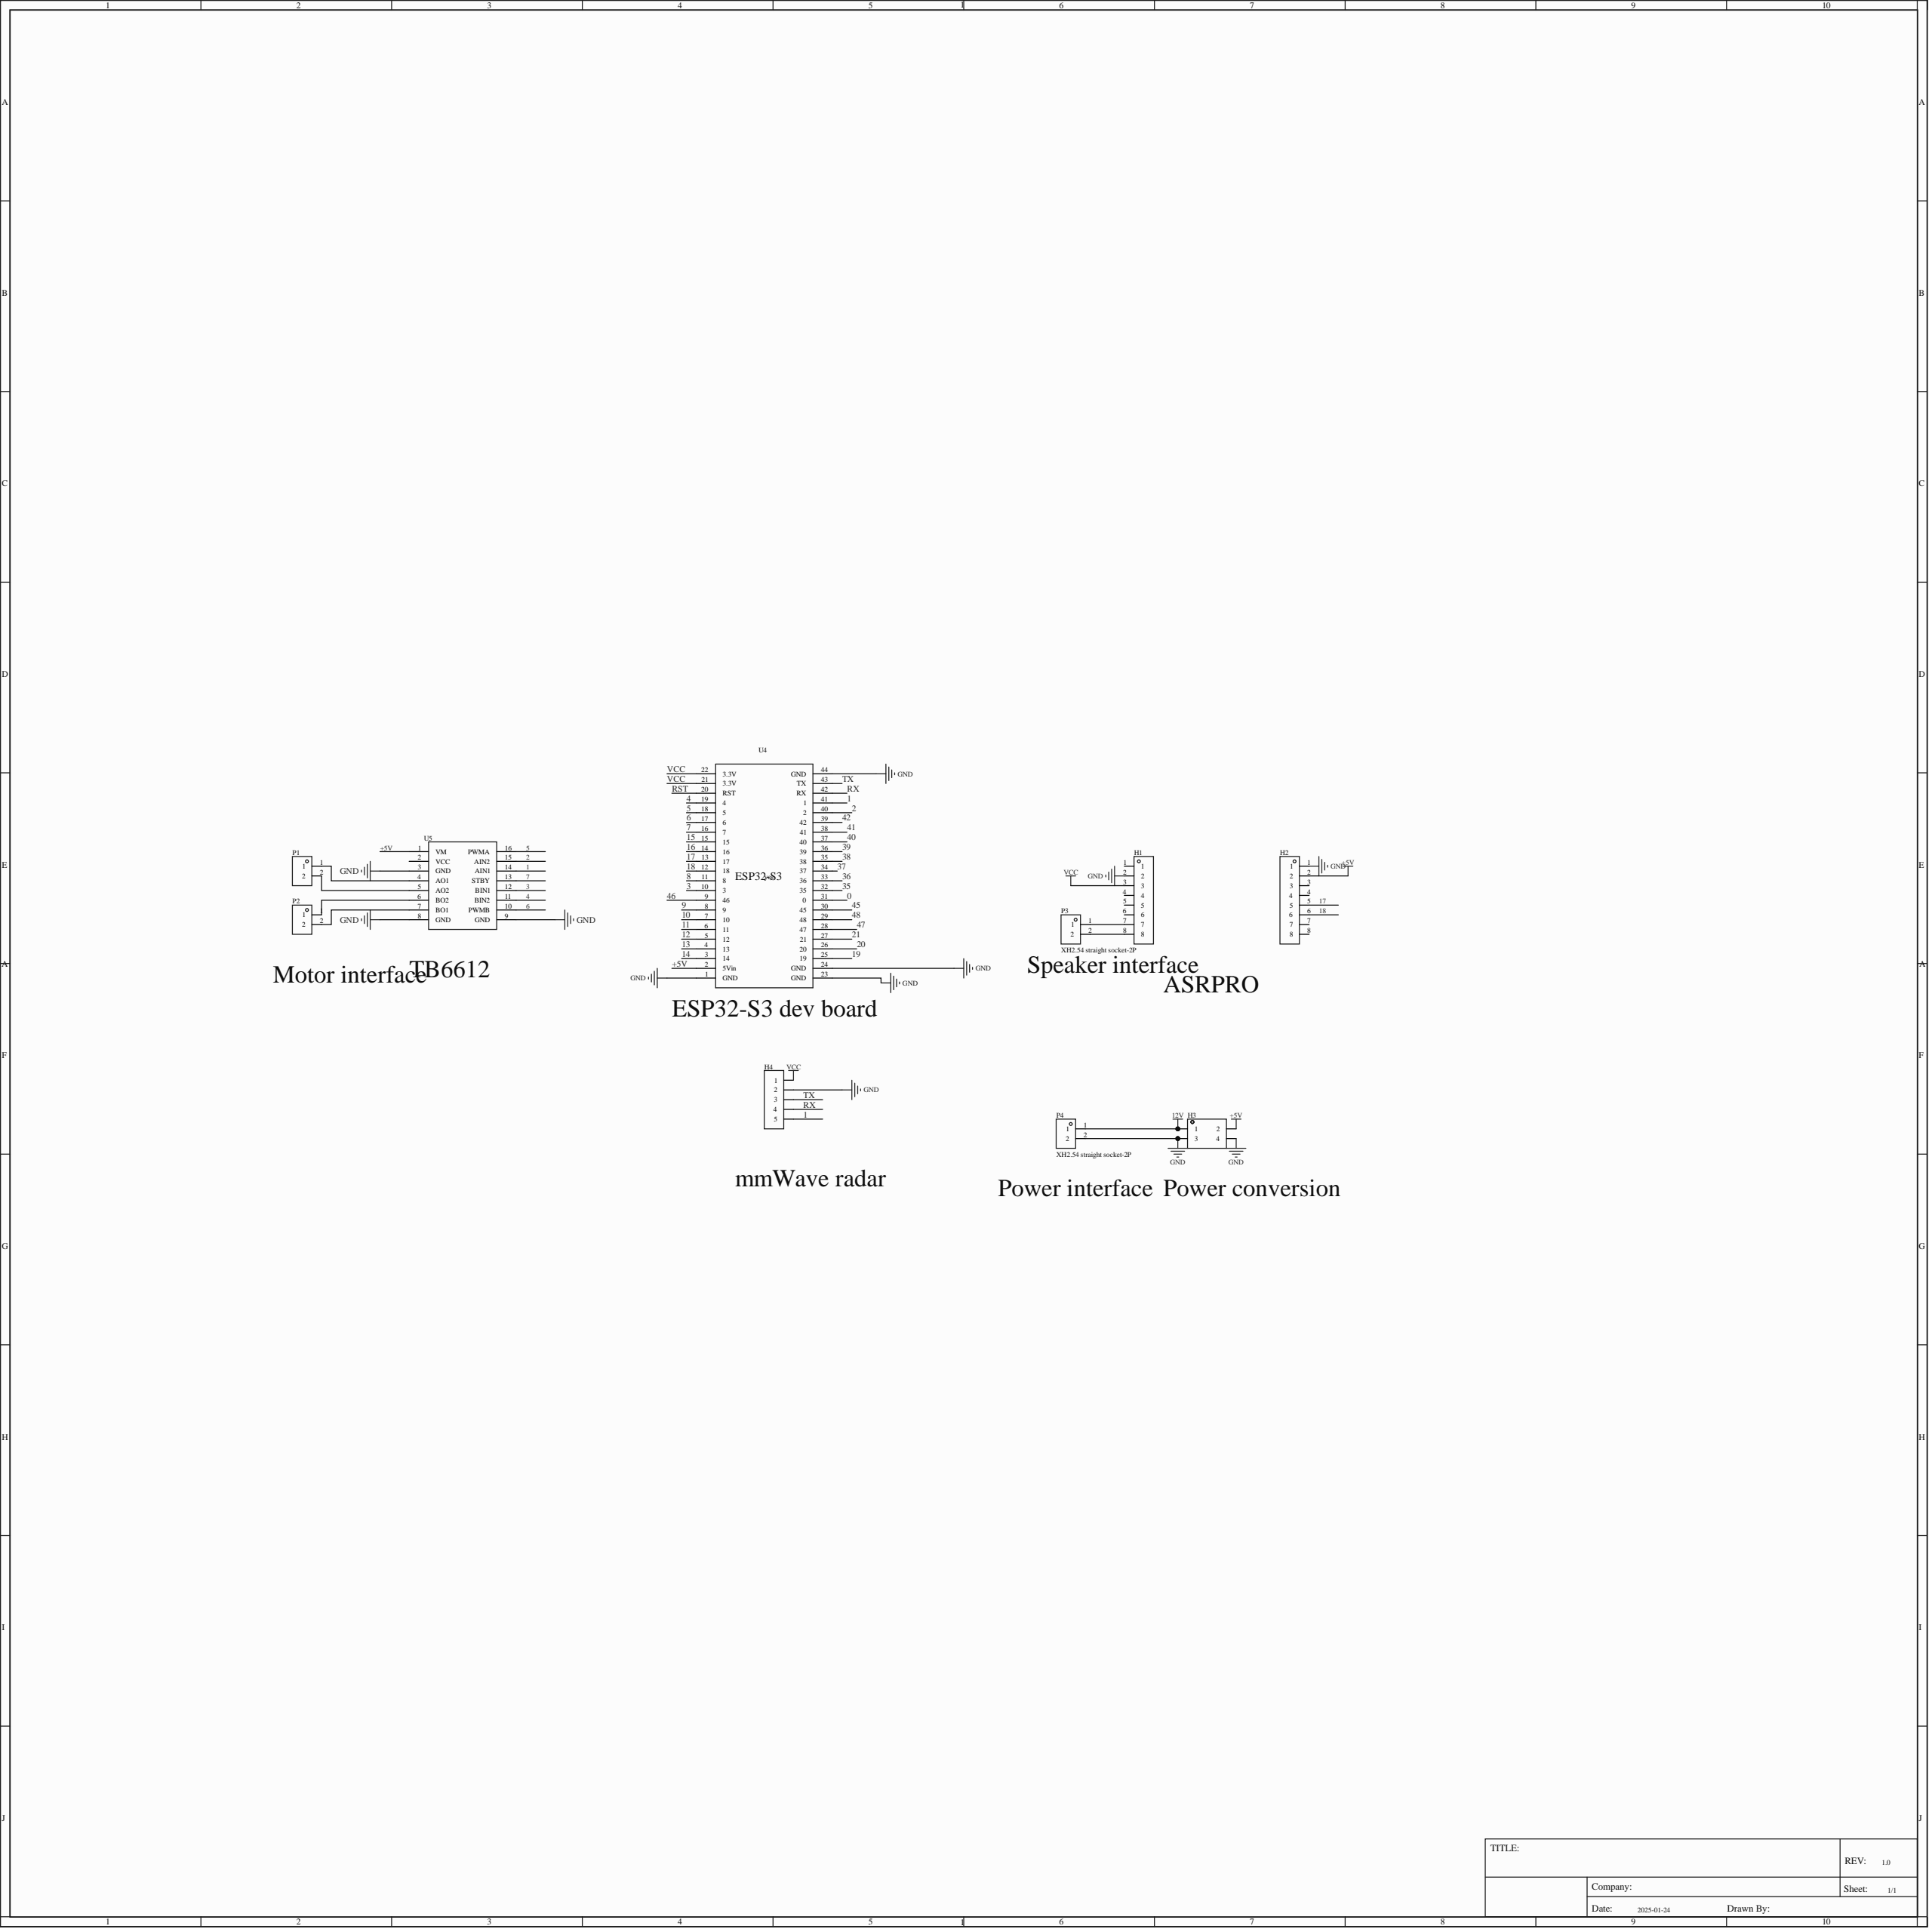Circuit board | Altium Designer | 10 parts | 21 nets
Bill of materials:
Comment,Description,Designator,Footprint,LibRef,Quantity
"","","H1, H2","HDR-TH_8P-P2.54-V-F-1","HDR-F_2.54_1x8P","2"
"","","H3","HDR-TH_4P-P2.54-V-F-R2-C2-S2.54","HDR-F_2.54_2x2","1"
"","","H4","HDR-TH_5P-P2.54-V-F","HDR-F_2.54_1x5P","1"
"KF301-2P terminal block","","P1, P2","CONN-TH_XY301V-A-5.0-2P","KF301-2P接线端子","2"
"XH2.54 straight socket-2P","","P3, P4","CONN-TH_XH2.54-2P","XH2.54直插座-2P","2"
"NO","","U4","ESP32S3","NO","1"
"","","U5","tb6612","tb6612","1"
Netlist (Protel format):
[
H1
HDR-TH_8P-P2.54-V-F-1




]
[
H2
HDR-TH_8P-P2.54-V-F-1




]
[
H3
HDR-TH_4P-P2.54-V-F-R2-C2-S2.54




]
[
H4
HDR-TH_5P-P2.54-V-F




]
[
P1
CONN-TH_XY301V-A-5.0-2P
KF301-2P terminal block



]
[
P2
CONN-TH_XY301V-A-5.0-2P
KF301-2P terminal block



]
[
P3
CONN-TH_XH2.54-2P
XH2.54 straight socket-2P



]
[
P4
CONN-TH_XH2.54-2P
XH2.54 straight socket-2P



]
[
U4
ESP32S3
NO



]
[
U5
tb6612




]
(
VCC
H1-3
H4-1
U4-21
U4-22
)
(
TX
H4-3
U4-43
)
(
RX
H4-4
U4-42
)
(
NetP2_2
P2-2
U5-7
)
(
NetP2_1
P2-1
U5-6
)
(
NetP1_2
P1-2
U5-5
)
(
NetP1_1
P1-1
U5-4
)
(
NetH1_8
H1-8
P3-2
)
(
NetH1_7
H1-7
P3-1
)
(
GND
H1-2
H2-1
H3-3
H3-4
H4-2
P4-2
U4-1
U4-23
U4-24
U4-44
U5-3
U5-8
U5-9
)
(
+5V
H2-2
H3-2
U4-2
U5-1
)
(
18
H2-6
U4-12
)
(
17
H2-5
U4-13
)
(
12V
H3-1
P4-1
)
(
7
U4-16
U5-13
)
(
6
U4-17
U5-10
)
(
5
U4-18
U5-16
)
(
4
U4-19
U5-11
)
(
3
U4-10
U5-12
)
(
2
U4-40
U5-15
)
(
1
H4-5
U4-41
U5-14
)